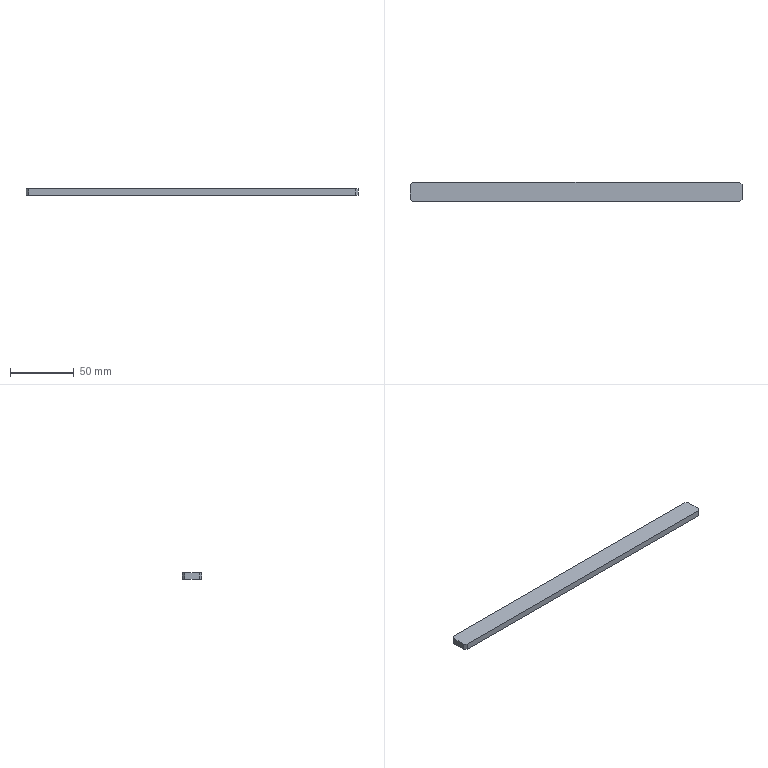Part | SolidWorks | features Chamfer 1, Extrusion 1 | 1 solid | 10 faces | box 260 x 15 x 5 mm | volume 19460 mm3 | plane 10
STEP:
#1=CARTESIAN_POINT('',(130.,-5.5,5.));
#2=VERTEX_POINT('',#1);
#3=CARTESIAN_POINT('',(130.,5.5,5.));
#4=VERTEX_POINT('',#3);
#5=CARTESIAN_POINT('',(130.,-7.5,5.));
#6=DIRECTION('',(0.,1.,0.));
#7=VECTOR('',#6,1000.);
#8=LINE('',#5,#7);
#9=EDGE_CURVE('',#2,#4,#8,.T.);
#10=ORIENTED_EDGE('',*,*,#9,.F.);
#11=CARTESIAN_POINT('',(130.,-5.5,0.));
#12=VERTEX_POINT('',#11);
#13=CARTESIAN_POINT('',(130.,-5.5,5.));
#14=DIRECTION('',(0.,0.,-1.));
#15=VECTOR('',#14,1000.);
#16=LINE('',#13,#15);
#17=EDGE_CURVE('',#2,#12,#16,.T.);
#18=ORIENTED_EDGE('',*,*,#17,.T.);
#19=CARTESIAN_POINT('',(130.,5.5,0.));
#20=VERTEX_POINT('',#19);
#21=CARTESIAN_POINT('',(130.,-7.5,0.));
#22=DIRECTION('',(0.,1.,0.));
#23=VECTOR('',#22,1000.);
#24=LINE('',#21,#23);
#25=EDGE_CURVE('',#12,#20,#24,.T.);
#26=ORIENTED_EDGE('',*,*,#25,.T.);
#27=CARTESIAN_POINT('',(130.,5.5,5.));
#28=DIRECTION('',(0.,0.,1.));
#29=VECTOR('',#28,1000.);
#30=LINE('',#27,#29);
#31=EDGE_CURVE('',#20,#4,#30,.T.);
#32=ORIENTED_EDGE('',*,*,#31,.T.);
#33=EDGE_LOOP('',(#10,#18,#26,#32));
#34=FACE_OUTER_BOUND('',#33,.T.);
#35=CARTESIAN_POINT('',(130.,-7.5,5.));
#36=DIRECTION('',(-1.,0.,0.));
#37=DIRECTION('',(0.,0.,1.));
#38=AXIS2_PLACEMENT_3D('',#35,#36,#37);
#39=PLANE('',#38);
#40=ADVANCED_FACE('',(#34),#39,.F.);
#41=CARTESIAN_POINT('',(128.,7.5,5.));
#42=VERTEX_POINT('',#41);
#43=CARTESIAN_POINT('',(-128.,7.5,5.));
#44=VERTEX_POINT('',#43);
#45=CARTESIAN_POINT('',(-130.,7.5,5.));
#46=DIRECTION('',(-1.,0.,0.));
#47=VECTOR('',#46,1000.);
#48=LINE('',#45,#47);
#49=EDGE_CURVE('',#42,#44,#48,.T.);
#50=ORIENTED_EDGE('',*,*,#49,.F.);
#51=CARTESIAN_POINT('',(128.,7.5,0.));
#52=VERTEX_POINT('',#51);
#53=CARTESIAN_POINT('',(128.,7.5,5.));
#54=DIRECTION('',(0.,0.,-1.));
#55=VECTOR('',#54,1000.);
#56=LINE('',#53,#55);
#57=EDGE_CURVE('',#42,#52,#56,.T.);
#58=ORIENTED_EDGE('',*,*,#57,.T.);
#59=CARTESIAN_POINT('',(-128.,7.5,0.));
#60=VERTEX_POINT('',#59);
#61=CARTESIAN_POINT('',(-130.,7.5,0.));
#62=DIRECTION('',(-1.,0.,0.));
#63=VECTOR('',#62,1000.);
#64=LINE('',#61,#63);
#65=EDGE_CURVE('',#52,#60,#64,.T.);
#66=ORIENTED_EDGE('',*,*,#65,.T.);
#67=CARTESIAN_POINT('',(-128.,7.5,5.));
#68=DIRECTION('',(0.,0.,1.));
#69=VECTOR('',#68,1000.);
#70=LINE('',#67,#69);
#71=EDGE_CURVE('',#60,#44,#70,.T.);
#72=ORIENTED_EDGE('',*,*,#71,.T.);
#73=EDGE_LOOP('',(#50,#58,#66,#72));
#74=FACE_OUTER_BOUND('',#73,.T.);
#75=CARTESIAN_POINT('',(-130.,7.5,5.));
#76=DIRECTION('',(0.,-1.,0.));
#77=DIRECTION('',(0.,0.,-1.));
#78=AXIS2_PLACEMENT_3D('',#75,#76,#77);
#79=PLANE('',#78);
#80=ADVANCED_FACE('',(#74),#79,.F.);
#81=CARTESIAN_POINT('',(-130.,5.5,0.));
#82=VERTEX_POINT('',#81);
#83=CARTESIAN_POINT('',(-130.,-5.5,0.));
#84=VERTEX_POINT('',#83);
#85=CARTESIAN_POINT('',(-130.,-7.5,0.));
#86=DIRECTION('',(0.,-1.,0.));
#87=VECTOR('',#86,1000.);
#88=LINE('',#85,#87);
#89=EDGE_CURVE('',#82,#84,#88,.T.);
#90=ORIENTED_EDGE('',*,*,#89,.T.);
#91=CARTESIAN_POINT('',(-130.,-5.5,5.));
#92=VERTEX_POINT('',#91);
#93=CARTESIAN_POINT('',(-130.,-5.5,5.));
#94=DIRECTION('',(0.,0.,1.));
#95=VECTOR('',#94,1000.);
#96=LINE('',#93,#95);
#97=EDGE_CURVE('',#84,#92,#96,.T.);
#98=ORIENTED_EDGE('',*,*,#97,.T.);
#99=CARTESIAN_POINT('',(-130.,5.5,5.));
#100=VERTEX_POINT('',#99);
#101=CARTESIAN_POINT('',(-130.,-7.5,5.));
#102=DIRECTION('',(0.,-1.,0.));
#103=VECTOR('',#102,1000.);
#104=LINE('',#101,#103);
#105=EDGE_CURVE('',#100,#92,#104,.T.);
#106=ORIENTED_EDGE('',*,*,#105,.F.);
#107=CARTESIAN_POINT('',(-130.,5.5,5.));
#108=DIRECTION('',(0.,0.,-1.));
#109=VECTOR('',#108,1000.);
#110=LINE('',#107,#109);
#111=EDGE_CURVE('',#100,#82,#110,.T.);
#112=ORIENTED_EDGE('',*,*,#111,.T.);
#113=EDGE_LOOP('',(#90,#98,#106,#112));
#114=FACE_OUTER_BOUND('',#113,.T.);
#115=CARTESIAN_POINT('',(-130.,-7.5,5.));
#116=DIRECTION('',(1.,0.,0.));
#117=DIRECTION('',(0.,0.,-1.));
#118=AXIS2_PLACEMENT_3D('',#115,#116,#117);
#119=PLANE('',#118);
#120=ADVANCED_FACE('',(#114),#119,.F.);
#121=CARTESIAN_POINT('',(-128.,-7.5,0.));
#122=VERTEX_POINT('',#121);
#123=CARTESIAN_POINT('',(128.,-7.5,0.));
#124=VERTEX_POINT('',#123);
#125=CARTESIAN_POINT('',(-130.,-7.5,0.));
#126=DIRECTION('',(1.,0.,0.));
#127=VECTOR('',#126,1000.);
#128=LINE('',#125,#127);
#129=EDGE_CURVE('',#122,#124,#128,.T.);
#130=ORIENTED_EDGE('',*,*,#129,.T.);
#131=CARTESIAN_POINT('',(128.,-7.5,5.));
#132=VERTEX_POINT('',#131);
#133=CARTESIAN_POINT('',(128.,-7.5,5.));
#134=DIRECTION('',(0.,0.,1.));
#135=VECTOR('',#134,1000.);
#136=LINE('',#133,#135);
#137=EDGE_CURVE('',#124,#132,#136,.T.);
#138=ORIENTED_EDGE('',*,*,#137,.T.);
#139=CARTESIAN_POINT('',(-128.,-7.5,5.));
#140=VERTEX_POINT('',#139);
#141=CARTESIAN_POINT('',(-130.,-7.5,5.));
#142=DIRECTION('',(1.,0.,0.));
#143=VECTOR('',#142,1000.);
#144=LINE('',#141,#143);
#145=EDGE_CURVE('',#140,#132,#144,.T.);
#146=ORIENTED_EDGE('',*,*,#145,.F.);
#147=CARTESIAN_POINT('',(-128.,-7.5,5.));
#148=DIRECTION('',(0.,0.,-1.));
#149=VECTOR('',#148,1000.);
#150=LINE('',#147,#149);
#151=EDGE_CURVE('',#140,#122,#150,.T.);
#152=ORIENTED_EDGE('',*,*,#151,.T.);
#153=EDGE_LOOP('',(#130,#138,#146,#152));
#154=FACE_OUTER_BOUND('',#153,.T.);
#155=CARTESIAN_POINT('',(-130.,-7.5,5.));
#156=DIRECTION('',(0.,1.,0.));
#157=DIRECTION('',(0.,0.,1.));
#158=AXIS2_PLACEMENT_3D('',#155,#156,#157);
#159=PLANE('',#158);
#160=ADVANCED_FACE('',(#154),#159,.F.);
#161=ORIENTED_EDGE('',*,*,#145,.T.);
#162=CARTESIAN_POINT('',(130.,-5.5,5.));
#163=DIRECTION('',(0.7071,0.7071,0.));
#164=VECTOR('',#163,1000.);
#165=LINE('',#162,#164);
#166=EDGE_CURVE('',#132,#2,#165,.T.);
#167=ORIENTED_EDGE('',*,*,#166,.T.);
#168=ORIENTED_EDGE('',*,*,#9,.T.);
#169=CARTESIAN_POINT('',(128.,7.5,5.));
#170=DIRECTION('',(-0.7071,0.7071,0.));
#171=VECTOR('',#170,1000.);
#172=LINE('',#169,#171);
#173=EDGE_CURVE('',#4,#42,#172,.T.);
#174=ORIENTED_EDGE('',*,*,#173,.T.);
#175=ORIENTED_EDGE('',*,*,#49,.T.);
#176=CARTESIAN_POINT('',(-130.,5.5,5.));
#177=DIRECTION('',(-0.7071,-0.7071,0.));
#178=VECTOR('',#177,1000.);
#179=LINE('',#176,#178);
#180=EDGE_CURVE('',#44,#100,#179,.T.);
#181=ORIENTED_EDGE('',*,*,#180,.T.);
#182=ORIENTED_EDGE('',*,*,#105,.T.);
#183=CARTESIAN_POINT('',(-128.,-7.5,5.));
#184=DIRECTION('',(0.7071,-0.7071,0.));
#185=VECTOR('',#184,1000.);
#186=LINE('',#183,#185);
#187=EDGE_CURVE('',#92,#140,#186,.T.);
#188=ORIENTED_EDGE('',*,*,#187,.T.);
#189=EDGE_LOOP('',(#161,#167,#168,#174,#175,#181,#182,#188));
#190=FACE_OUTER_BOUND('',#189,.T.);
#191=CARTESIAN_POINT('',(0.,0.,5.));
#192=DIRECTION('',(0.,0.,-1.));
#193=DIRECTION('',(-1.,0.,0.));
#194=AXIS2_PLACEMENT_3D('',#191,#192,#193);
#195=PLANE('',#194);
#196=ADVANCED_FACE('',(#190),#195,.F.);
#197=ORIENTED_EDGE('',*,*,#25,.F.);
#198=CARTESIAN_POINT('',(67.75,-67.75,0.));
#199=DIRECTION('',(-0.7071,-0.7071,0.));
#200=VECTOR('',#199,1000.);
#201=LINE('',#198,#200);
#202=EDGE_CURVE('',#12,#124,#201,.T.);
#203=ORIENTED_EDGE('',*,*,#202,.T.);
#204=ORIENTED_EDGE('',*,*,#129,.F.);
#205=CARTESIAN_POINT('',(-67.75,-67.75,0.));
#206=DIRECTION('',(-0.7071,0.7071,0.));
#207=VECTOR('',#206,1000.);
#208=LINE('',#205,#207);
#209=EDGE_CURVE('',#122,#84,#208,.T.);
#210=ORIENTED_EDGE('',*,*,#209,.T.);
#211=ORIENTED_EDGE('',*,*,#89,.F.);
#212=CARTESIAN_POINT('',(-67.75,67.75,0.));
#213=DIRECTION('',(0.7071,0.7071,0.));
#214=VECTOR('',#213,1000.);
#215=LINE('',#212,#214);
#216=EDGE_CURVE('',#82,#60,#215,.T.);
#217=ORIENTED_EDGE('',*,*,#216,.T.);
#218=ORIENTED_EDGE('',*,*,#65,.F.);
#219=CARTESIAN_POINT('',(67.75,67.75,0.));
#220=DIRECTION('',(0.7071,-0.7071,0.));
#221=VECTOR('',#220,1000.);
#222=LINE('',#219,#221);
#223=EDGE_CURVE('',#52,#20,#222,.T.);
#224=ORIENTED_EDGE('',*,*,#223,.T.);
#225=EDGE_LOOP('',(#197,#203,#204,#210,#211,#217,#218,#224));
#226=FACE_OUTER_BOUND('',#225,.T.);
#227=CARTESIAN_POINT('',(0.,0.,0.));
#228=DIRECTION('',(0.,0.,-1.));
#229=DIRECTION('',(-1.,0.,0.));
#230=AXIS2_PLACEMENT_3D('',#227,#228,#229);
#231=PLANE('',#230);
#232=ADVANCED_FACE('',(#226),#231,.T.);
#233=ORIENTED_EDGE('',*,*,#166,.F.);
#234=ORIENTED_EDGE('',*,*,#137,.F.);
#235=ORIENTED_EDGE('',*,*,#202,.F.);
#236=ORIENTED_EDGE('',*,*,#17,.F.);
#237=EDGE_LOOP('',(#233,#234,#235,#236));
#238=FACE_OUTER_BOUND('',#237,.T.);
#239=CARTESIAN_POINT('',(130.,-5.5,5.));
#240=DIRECTION('',(-0.7071,0.7071,0.));
#241=DIRECTION('',(0.,0.,-1.));
#242=AXIS2_PLACEMENT_3D('',#239,#240,#241);
#243=PLANE('',#242);
#244=ADVANCED_FACE('',(#238),#243,.F.);
#245=ORIENTED_EDGE('',*,*,#173,.F.);
#246=ORIENTED_EDGE('',*,*,#31,.F.);
#247=ORIENTED_EDGE('',*,*,#223,.F.);
#248=ORIENTED_EDGE('',*,*,#57,.F.);
#249=EDGE_LOOP('',(#245,#246,#247,#248));
#250=FACE_OUTER_BOUND('',#249,.T.);
#251=CARTESIAN_POINT('',(128.,7.5,5.));
#252=DIRECTION('',(-0.7071,-0.7071,0.));
#253=DIRECTION('',(0.,0.,-1.));
#254=AXIS2_PLACEMENT_3D('',#251,#252,#253);
#255=PLANE('',#254);
#256=ADVANCED_FACE('',(#250),#255,.F.);
#257=ORIENTED_EDGE('',*,*,#187,.F.);
#258=ORIENTED_EDGE('',*,*,#97,.F.);
#259=ORIENTED_EDGE('',*,*,#209,.F.);
#260=ORIENTED_EDGE('',*,*,#151,.F.);
#261=EDGE_LOOP('',(#257,#258,#259,#260));
#262=FACE_OUTER_BOUND('',#261,.T.);
#263=CARTESIAN_POINT('',(-128.,-7.5,5.));
#264=DIRECTION('',(0.7071,0.7071,0.));
#265=DIRECTION('',(0.,0.,-1.));
#266=AXIS2_PLACEMENT_3D('',#263,#264,#265);
#267=PLANE('',#266);
#268=ADVANCED_FACE('',(#262),#267,.F.);
#269=ORIENTED_EDGE('',*,*,#180,.F.);
#270=ORIENTED_EDGE('',*,*,#71,.F.);
#271=ORIENTED_EDGE('',*,*,#216,.F.);
#272=ORIENTED_EDGE('',*,*,#111,.F.);
#273=EDGE_LOOP('',(#269,#270,#271,#272));
#274=FACE_OUTER_BOUND('',#273,.T.);
#275=CARTESIAN_POINT('',(-130.,5.5,5.));
#276=DIRECTION('',(0.7071,-0.7071,0.));
#277=DIRECTION('',(0.,0.,-1.));
#278=AXIS2_PLACEMENT_3D('',#275,#276,#277);
#279=PLANE('',#278);
#280=ADVANCED_FACE('',(#274),#279,.F.);
#281=CLOSED_SHELL('',(#40,#80,#120,#160,#196,#232,#244,#256,#268,#280));
#282=MANIFOLD_SOLID_BREP('',#281);
#283=CARTESIAN_POINT('',(0.,0.,0.));
#284=DIRECTION('',(0.,0.,1.));
#285=DIRECTION('',(1.,0.,0.));
#286=AXIS2_PLACEMENT_3D('',#283,#284,#285);
#287=(LENGTH_UNIT()NAMED_UNIT(*)SI_UNIT(.MILLI.,.METRE.));
#288=UNCERTAINTY_MEASURE_WITH_UNIT(LENGTH_MEASURE(0.00001),#287,'','');
#289=(NAMED_UNIT(*)PLANE_ANGLE_UNIT()SI_UNIT($,.RADIAN.));
#290=(NAMED_UNIT(*)SI_UNIT($,.STERADIAN.)SOLID_ANGLE_UNIT());
#291=(GEOMETRIC_REPRESENTATION_CONTEXT(3)GLOBAL_UNCERTAINTY_ASSIGNED_CONTEXT((#288))GLOBAL_UNIT_ASSIGNED_CONTEXT((#287,#289,#290))REPRESENTATION_CONTEXT('',''));
#292=ADVANCED_BREP_SHAPE_REPRESENTATION('',(#282,#286),#291);